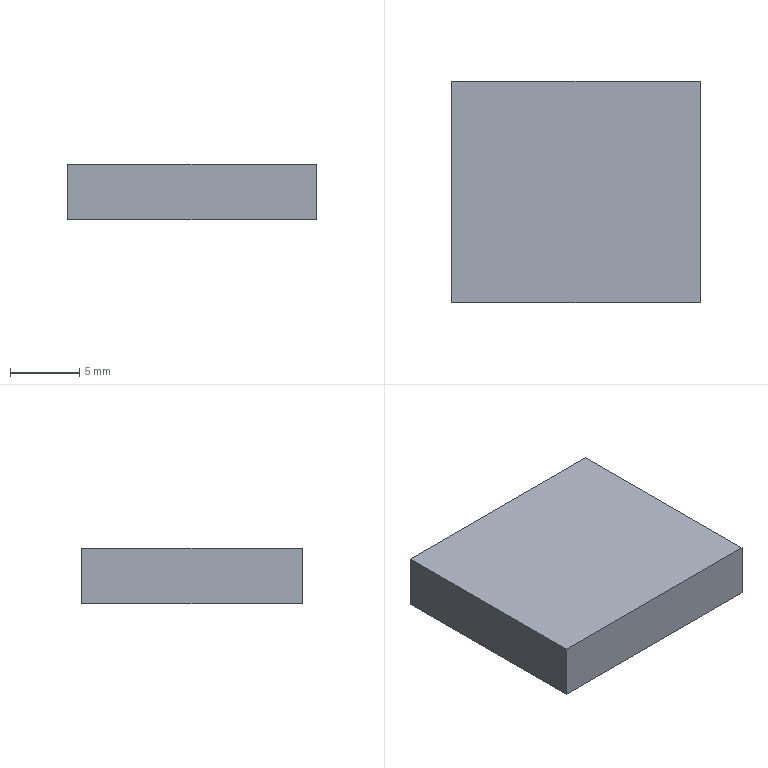Part | SolidWorks | features BaseBody 1 | 1 solid | 6 faces | box 18 x 16 x 4 mm | volume 1152 mm3 | plane 6
STEP:
#1=CARTESIAN_POINT('',(9.,-8.,0.));
#2=VERTEX_POINT('',#1);
#3=CARTESIAN_POINT('',(9.,8.,0.));
#4=VERTEX_POINT('',#3);
#5=CARTESIAN_POINT('',(9.,-8.,0.));
#6=DIRECTION('',(0.,1.,0.));
#7=VECTOR('',#6,1000.);
#8=LINE('',#5,#7);
#9=EDGE_CURVE('',#2,#4,#8,.T.);
#10=ORIENTED_EDGE('',*,*,#9,.F.);
#11=CARTESIAN_POINT('',(-9.,-8.,0.));
#12=VERTEX_POINT('',#11);
#13=CARTESIAN_POINT('',(-9.,-8.,0.));
#14=DIRECTION('',(1.,0.,0.));
#15=VECTOR('',#14,1000.);
#16=LINE('',#13,#15);
#17=EDGE_CURVE('',#12,#2,#16,.T.);
#18=ORIENTED_EDGE('',*,*,#17,.F.);
#19=CARTESIAN_POINT('',(-9.,8.,0.));
#20=VERTEX_POINT('',#19);
#21=CARTESIAN_POINT('',(-9.,-8.,0.));
#22=DIRECTION('',(0.,-1.,0.));
#23=VECTOR('',#22,1000.);
#24=LINE('',#21,#23);
#25=EDGE_CURVE('',#20,#12,#24,.T.);
#26=ORIENTED_EDGE('',*,*,#25,.F.);
#27=CARTESIAN_POINT('',(-9.,8.,0.));
#28=DIRECTION('',(-1.,0.,0.));
#29=VECTOR('',#28,1000.);
#30=LINE('',#27,#29);
#31=EDGE_CURVE('',#4,#20,#30,.T.);
#32=ORIENTED_EDGE('',*,*,#31,.F.);
#33=EDGE_LOOP('',(#10,#18,#26,#32));
#34=FACE_OUTER_BOUND('',#33,.T.);
#35=CARTESIAN_POINT('',(-9.,-8.,0.));
#36=DIRECTION('',(0.,0.,1.));
#37=DIRECTION('',(1.,0.,0.));
#38=AXIS2_PLACEMENT_3D('',#35,#36,#37);
#39=PLANE('',#38);
#40=ADVANCED_FACE('',(#34),#39,.F.);
#41=CARTESIAN_POINT('',(-9.,8.,4.));
#42=VERTEX_POINT('',#41);
#43=CARTESIAN_POINT('',(9.,8.,4.));
#44=VERTEX_POINT('',#43);
#45=CARTESIAN_POINT('',(-9.,8.,4.));
#46=DIRECTION('',(1.,0.,0.));
#47=VECTOR('',#46,1000.);
#48=LINE('',#45,#47);
#49=EDGE_CURVE('',#42,#44,#48,.T.);
#50=ORIENTED_EDGE('',*,*,#49,.T.);
#51=CARTESIAN_POINT('',(9.,8.,0.));
#52=DIRECTION('',(0.,0.,-1.));
#53=VECTOR('',#52,1000.);
#54=LINE('',#51,#53);
#55=EDGE_CURVE('',#44,#4,#54,.T.);
#56=ORIENTED_EDGE('',*,*,#55,.T.);
#57=ORIENTED_EDGE('',*,*,#31,.T.);
#58=CARTESIAN_POINT('',(-9.,8.,0.));
#59=DIRECTION('',(0.,0.,1.));
#60=VECTOR('',#59,1000.);
#61=LINE('',#58,#60);
#62=EDGE_CURVE('',#20,#42,#61,.T.);
#63=ORIENTED_EDGE('',*,*,#62,.T.);
#64=EDGE_LOOP('',(#50,#56,#57,#63));
#65=FACE_OUTER_BOUND('',#64,.T.);
#66=CARTESIAN_POINT('',(-9.,8.,0.));
#67=DIRECTION('',(0.,1.,0.));
#68=DIRECTION('',(0.,0.,1.));
#69=AXIS2_PLACEMENT_3D('',#66,#67,#68);
#70=PLANE('',#69);
#71=ADVANCED_FACE('',(#65),#70,.T.);
#72=ORIENTED_EDGE('',*,*,#55,.F.);
#73=CARTESIAN_POINT('',(9.,-8.,4.));
#74=VERTEX_POINT('',#73);
#75=CARTESIAN_POINT('',(9.,-8.,4.));
#76=DIRECTION('',(0.,-1.,0.));
#77=VECTOR('',#76,1000.);
#78=LINE('',#75,#77);
#79=EDGE_CURVE('',#44,#74,#78,.T.);
#80=ORIENTED_EDGE('',*,*,#79,.T.);
#81=CARTESIAN_POINT('',(9.,-8.,0.));
#82=DIRECTION('',(0.,0.,-1.));
#83=VECTOR('',#82,1000.);
#84=LINE('',#81,#83);
#85=EDGE_CURVE('',#74,#2,#84,.T.);
#86=ORIENTED_EDGE('',*,*,#85,.T.);
#87=ORIENTED_EDGE('',*,*,#9,.T.);
#88=EDGE_LOOP('',(#72,#80,#86,#87));
#89=FACE_OUTER_BOUND('',#88,.T.);
#90=CARTESIAN_POINT('',(9.,-8.,0.));
#91=DIRECTION('',(1.,0.,0.));
#92=DIRECTION('',(0.,0.,-1.));
#93=AXIS2_PLACEMENT_3D('',#90,#91,#92);
#94=PLANE('',#93);
#95=ADVANCED_FACE('',(#89),#94,.T.);
#96=CARTESIAN_POINT('',(-9.,-8.,4.));
#97=VERTEX_POINT('',#96);
#98=CARTESIAN_POINT('',(-9.,-8.,4.));
#99=DIRECTION('',(1.,0.,0.));
#100=VECTOR('',#99,1000.);
#101=LINE('',#98,#100);
#102=EDGE_CURVE('',#97,#74,#101,.T.);
#103=ORIENTED_EDGE('',*,*,#102,.F.);
#104=CARTESIAN_POINT('',(-9.,-8.,0.));
#105=DIRECTION('',(0.,0.,1.));
#106=VECTOR('',#105,1000.);
#107=LINE('',#104,#106);
#108=EDGE_CURVE('',#12,#97,#107,.T.);
#109=ORIENTED_EDGE('',*,*,#108,.F.);
#110=ORIENTED_EDGE('',*,*,#17,.T.);
#111=ORIENTED_EDGE('',*,*,#85,.F.);
#112=EDGE_LOOP('',(#103,#109,#110,#111));
#113=FACE_OUTER_BOUND('',#112,.T.);
#114=CARTESIAN_POINT('',(-9.,-8.,0.));
#115=DIRECTION('',(0.,1.,0.));
#116=DIRECTION('',(0.,0.,1.));
#117=AXIS2_PLACEMENT_3D('',#114,#115,#116);
#118=PLANE('',#117);
#119=ADVANCED_FACE('',(#113),#118,.F.);
#120=ORIENTED_EDGE('',*,*,#62,.F.);
#121=ORIENTED_EDGE('',*,*,#25,.T.);
#122=ORIENTED_EDGE('',*,*,#108,.T.);
#123=CARTESIAN_POINT('',(-9.,-8.,4.));
#124=DIRECTION('',(0.,-1.,0.));
#125=VECTOR('',#124,1000.);
#126=LINE('',#123,#125);
#127=EDGE_CURVE('',#42,#97,#126,.T.);
#128=ORIENTED_EDGE('',*,*,#127,.F.);
#129=EDGE_LOOP('',(#120,#121,#122,#128));
#130=FACE_OUTER_BOUND('',#129,.T.);
#131=CARTESIAN_POINT('',(-9.,-8.,0.));
#132=DIRECTION('',(1.,0.,0.));
#133=DIRECTION('',(0.,0.,-1.));
#134=AXIS2_PLACEMENT_3D('',#131,#132,#133);
#135=PLANE('',#134);
#136=ADVANCED_FACE('',(#130),#135,.F.);
#137=ORIENTED_EDGE('',*,*,#79,.F.);
#138=ORIENTED_EDGE('',*,*,#49,.F.);
#139=ORIENTED_EDGE('',*,*,#127,.T.);
#140=ORIENTED_EDGE('',*,*,#102,.T.);
#141=EDGE_LOOP('',(#137,#138,#139,#140));
#142=FACE_OUTER_BOUND('',#141,.T.);
#143=CARTESIAN_POINT('',(-9.,-8.,4.));
#144=DIRECTION('',(0.,0.,1.));
#145=DIRECTION('',(1.,0.,0.));
#146=AXIS2_PLACEMENT_3D('',#143,#144,#145);
#147=PLANE('',#146);
#148=ADVANCED_FACE('',(#142),#147,.T.);
#149=CLOSED_SHELL('',(#40,#71,#95,#119,#136,#148));
#150=MANIFOLD_SOLID_BREP('',#149);
#151=CARTESIAN_POINT('',(0.,0.,0.));
#152=DIRECTION('',(0.,0.,1.));
#153=DIRECTION('',(1.,0.,0.));
#154=AXIS2_PLACEMENT_3D('',#151,#152,#153);
#155=(LENGTH_UNIT()NAMED_UNIT(*)SI_UNIT(.MILLI.,.METRE.));
#156=UNCERTAINTY_MEASURE_WITH_UNIT(LENGTH_MEASURE(0.00001),#155,'','');
#157=(NAMED_UNIT(*)PLANE_ANGLE_UNIT()SI_UNIT($,.RADIAN.));
#158=(NAMED_UNIT(*)SI_UNIT($,.STERADIAN.)SOLID_ANGLE_UNIT());
#159=(GEOMETRIC_REPRESENTATION_CONTEXT(3)GLOBAL_UNCERTAINTY_ASSIGNED_CONTEXT((#156))GLOBAL_UNIT_ASSIGNED_CONTEXT((#155,#157,#158))REPRESENTATION_CONTEXT('',''));
#160=ADVANCED_BREP_SHAPE_REPRESENTATION('',(#150,#154),#159);